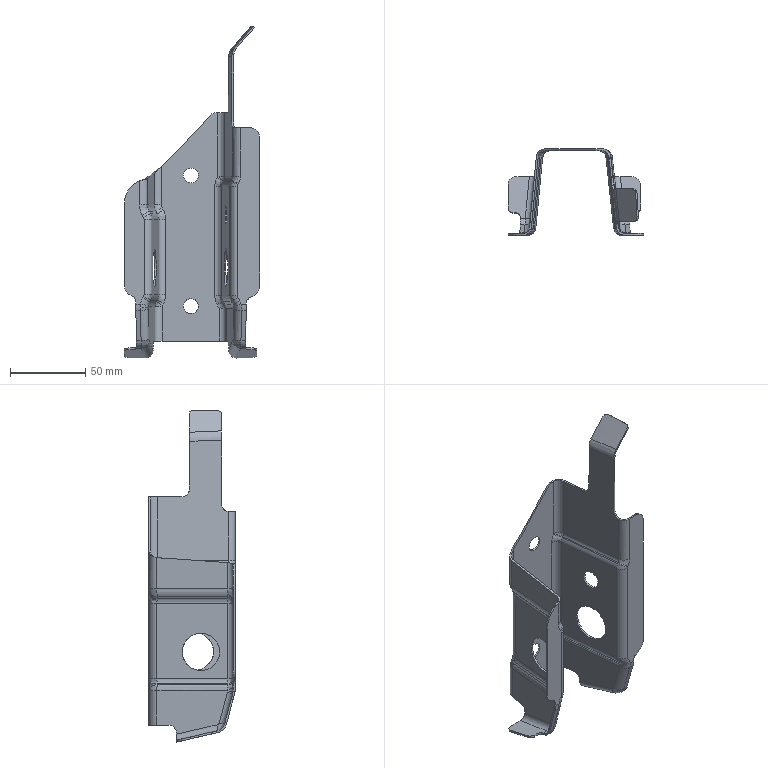Part | STEP file | FNA5401275 | 1 solid | 242 faces | box 90 x 57.5 x 220.985 mm | volume 30019 mm3 | spline 106 | cylinder 71 | plane 49 | other 16 | commonest cylinder face diameters 12 x17 8 x12 10.4 x12 9.6 x10 10 x6 25 x4